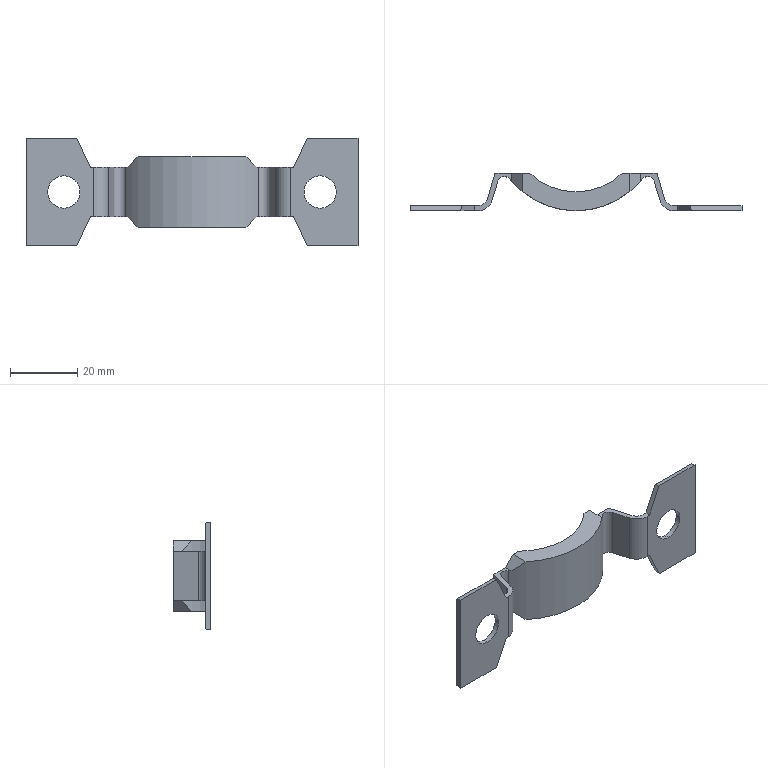Part | SolidWorks | features BaseBody 1 | 1 solid | 49 faces | box 98.5 x 11.15 x 32 mm | volume 4749 mm3 | plane 30 | cylinder 13 | sphere 2 | cone 2 | torus 2 | commonest cylinder face diameters 9.6 x4 4 x2 6 x2 9 x2 39.419 x2 50.6 x1